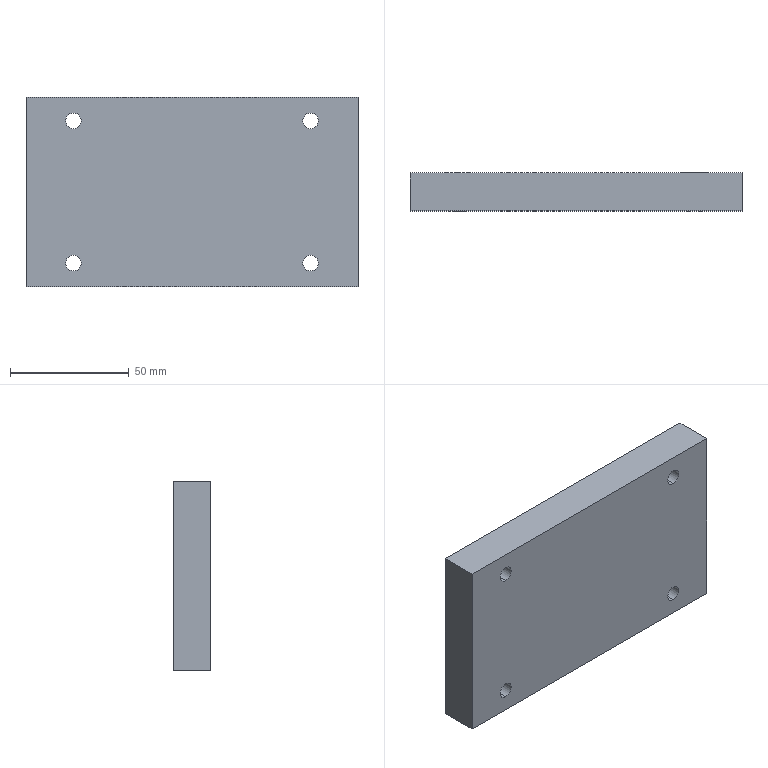Part | STEP file | 1 solid | 26 faces | box 140 x 16 x 80 mm | volume 175356 mm3 | cylinder 16 | plane 10 | commonest cylinder face diameters 6.6 x8 11 x8